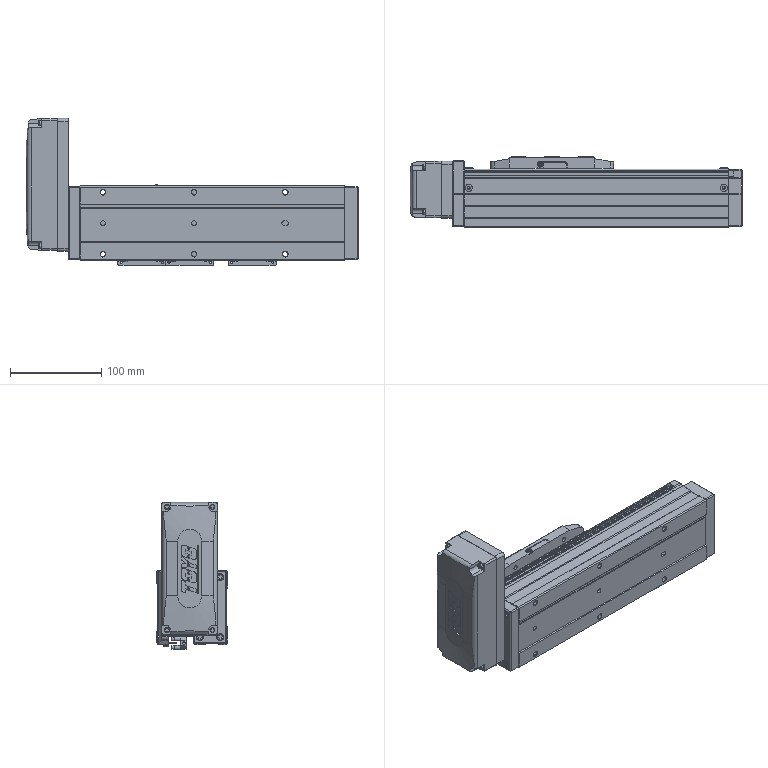Part | SolidWorks | features BaseBody 14 | 14 solids | 1494 faces | box 364.5 x 78 x 161.5 mm | volume 1915592 mm3 | plane 957 | cylinder 403 | cone 74 | torus 60 | commonest cylinder face diameters 1 x40 5.5 x40 2 x36 8 x32 7 x28 4 x27